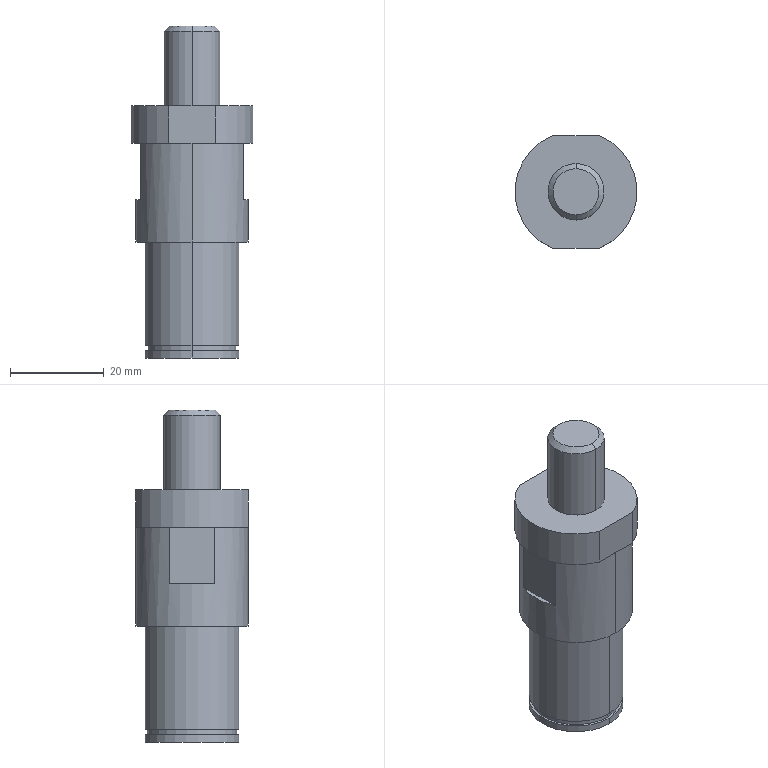Part | STEP file | TNSN20-Y20-F22-Part-2-1 | 1 solid | 28 faces | box 26 x 24 x 70.7 mm | volume 23111 mm3 | plane 14 | cylinder 12 | cone 2 | commonest cylinder face diameters 20 x4 12 x2 19 x2 24 x2 26 x2
STEP:
#1=CARTESIAN_POINT('',(14072.745,13708.046,9.));
#2=VERTEX_POINT('',#1);
#3=CARTESIAN_POINT('',(14072.745,13732.046,9.));
#4=VERTEX_POINT('',#3);
#5=CARTESIAN_POINT('',(14077.745,13720.046,9.));
#6=DIRECTION('',(0.,0.,-1.));
#7=DIRECTION('',(-0.3846,-0.9231,0.));
#8=AXIS2_PLACEMENT_3D('',#5,#6,#7);
#9=CIRCLE('',#8,13.);
#10=EDGE_CURVE('',#2,#4,#9,.T.);
#11=ORIENTED_EDGE('',*,*,#10,.F.);
#12=CARTESIAN_POINT('',(14082.745,13708.046,9.));
#13=VERTEX_POINT('',#12);
#14=CARTESIAN_POINT('',(14082.745,13708.046,9.));
#15=DIRECTION('',(-1.,0.,0.));
#16=VECTOR('',#15,1000.);
#17=LINE('',#14,#16);
#18=EDGE_CURVE('',#13,#2,#17,.T.);
#19=ORIENTED_EDGE('',*,*,#18,.F.);
#20=CARTESIAN_POINT('',(14082.745,13732.046,9.));
#21=VERTEX_POINT('',#20);
#22=CARTESIAN_POINT('',(14077.745,13720.046,9.));
#23=DIRECTION('',(0.,0.,-1.));
#24=DIRECTION('',(0.3846,0.9231,0.));
#25=AXIS2_PLACEMENT_3D('',#22,#23,#24);
#26=CIRCLE('',#25,13.);
#27=EDGE_CURVE('',#21,#13,#26,.T.);
#28=ORIENTED_EDGE('',*,*,#27,.F.);
#29=CARTESIAN_POINT('',(14072.745,13732.046,9.));
#30=DIRECTION('',(1.,0.,0.));
#31=VECTOR('',#30,1000.);
#32=LINE('',#29,#31);
#33=EDGE_CURVE('',#4,#21,#32,.T.);
#34=ORIENTED_EDGE('',*,*,#33,.F.);
#35=EDGE_LOOP('',(#11,#19,#28,#34));
#36=FACE_OUTER_BOUND('',#35,.T.);
#37=CARTESIAN_POINT('',(14077.745,13714.046,9.));
#38=VERTEX_POINT('',#37);
#39=CARTESIAN_POINT('',(14077.745,13726.046,9.));
#40=VERTEX_POINT('',#39);
#41=CARTESIAN_POINT('',(14077.745,13720.046,9.));
#42=DIRECTION('',(0.,0.,-1.));
#43=DIRECTION('',(0.,-1.,0.));
#44=AXIS2_PLACEMENT_3D('',#41,#42,#43);
#45=CIRCLE('',#44,6.);
#46=EDGE_CURVE('',#38,#40,#45,.T.);
#47=ORIENTED_EDGE('',*,*,#46,.T.);
#48=CARTESIAN_POINT('',(14077.745,13720.046,9.));
#49=DIRECTION('',(0.,0.,-1.));
#50=DIRECTION('',(0.,-1.,0.));
#51=AXIS2_PLACEMENT_3D('',#48,#49,#50);
#52=CIRCLE('',#51,6.);
#53=EDGE_CURVE('',#40,#38,#52,.T.);
#54=ORIENTED_EDGE('',*,*,#53,.T.);
#55=EDGE_LOOP('',(#47,#54));
#56=FACE_BOUND('',#55,.T.);
#57=CARTESIAN_POINT('',(14104.283,13746.584,9.));
#58=DIRECTION('',(0.,0.,-1.));
#59=DIRECTION('',(0.,-1.,0.));
#60=AXIS2_PLACEMENT_3D('',#57,#58,#59);
#61=PLANE('',#60);
#62=ADVANCED_FACE('',(#36,#56),#61,.F.);
#63=CARTESIAN_POINT('',(14082.745,13708.046,1.));
#64=VERTEX_POINT('',#63);
#65=CARTESIAN_POINT('',(14082.745,13708.046,9.));
#66=DIRECTION('',(0.,0.,-1.));
#67=VECTOR('',#66,1000.);
#68=LINE('',#65,#67);
#69=EDGE_CURVE('',#13,#64,#68,.T.);
#70=ORIENTED_EDGE('',*,*,#69,.T.);
#71=CARTESIAN_POINT('',(14082.745,13732.046,1.));
#72=VERTEX_POINT('',#71);
#73=CARTESIAN_POINT('',(14077.745,13720.046,1.));
#74=DIRECTION('',(0.,0.,-1.));
#75=DIRECTION('',(0.3846,0.9231,0.));
#76=AXIS2_PLACEMENT_3D('',#73,#74,#75);
#77=CIRCLE('',#76,13.);
#78=EDGE_CURVE('',#72,#64,#77,.T.);
#79=ORIENTED_EDGE('',*,*,#78,.F.);
#80=CARTESIAN_POINT('',(14082.745,13732.046,9.));
#81=DIRECTION('',(0.,0.,-1.));
#82=VECTOR('',#81,1000.);
#83=LINE('',#80,#82);
#84=EDGE_CURVE('',#21,#72,#83,.T.);
#85=ORIENTED_EDGE('',*,*,#84,.F.);
#86=ORIENTED_EDGE('',*,*,#27,.T.);
#87=EDGE_LOOP('',(#70,#79,#85,#86));
#88=FACE_OUTER_BOUND('',#87,.T.);
#89=CARTESIAN_POINT('',(14077.745,13720.046,5.));
#90=DIRECTION('',(0.,0.,-1.));
#91=DIRECTION('',(0.,-1.,0.));
#92=AXIS2_PLACEMENT_3D('',#89,#90,#91);
#93=CYLINDRICAL_SURFACE('',#92,13.);
#94=ADVANCED_FACE('',(#88),#93,.T.);
#95=CARTESIAN_POINT('',(14072.745,13732.046,1.));
#96=VERTEX_POINT('',#95);
#97=CARTESIAN_POINT('',(14072.745,13732.046,9.));
#98=DIRECTION('',(0.,0.,-1.));
#99=VECTOR('',#98,1000.);
#100=LINE('',#97,#99);
#101=EDGE_CURVE('',#4,#96,#100,.T.);
#102=ORIENTED_EDGE('',*,*,#101,.T.);
#103=CARTESIAN_POINT('',(14072.745,13708.046,1.));
#104=VERTEX_POINT('',#103);
#105=CARTESIAN_POINT('',(14077.745,13720.046,1.));
#106=DIRECTION('',(0.,0.,-1.));
#107=DIRECTION('',(-0.3846,-0.9231,0.));
#108=AXIS2_PLACEMENT_3D('',#105,#106,#107);
#109=CIRCLE('',#108,13.);
#110=EDGE_CURVE('',#104,#96,#109,.T.);
#111=ORIENTED_EDGE('',*,*,#110,.F.);
#112=CARTESIAN_POINT('',(14072.745,13708.046,9.));
#113=DIRECTION('',(0.,0.,-1.));
#114=VECTOR('',#113,1000.);
#115=LINE('',#112,#114);
#116=EDGE_CURVE('',#2,#104,#115,.T.);
#117=ORIENTED_EDGE('',*,*,#116,.F.);
#118=ORIENTED_EDGE('',*,*,#10,.T.);
#119=EDGE_LOOP('',(#102,#111,#117,#118));
#120=FACE_OUTER_BOUND('',#119,.T.);
#121=CARTESIAN_POINT('',(14077.745,13720.046,5.));
#122=DIRECTION('',(0.,0.,-1.));
#123=DIRECTION('',(0.,-1.,0.));
#124=AXIS2_PLACEMENT_3D('',#121,#122,#123);
#125=CYLINDRICAL_SURFACE('',#124,13.);
#126=ADVANCED_FACE('',(#120),#125,.T.);
#127=ORIENTED_EDGE('',*,*,#78,.T.);
#128=CARTESIAN_POINT('',(14077.745,13708.046,1.));
#129=VERTEX_POINT('',#128);
#130=CARTESIAN_POINT('',(14082.745,13708.046,1.));
#131=DIRECTION('',(-1.,0.,0.));
#132=VECTOR('',#131,1000.);
#133=LINE('',#130,#132);
#134=EDGE_CURVE('',#64,#129,#133,.T.);
#135=ORIENTED_EDGE('',*,*,#134,.T.);
#136=CARTESIAN_POINT('',(14088.745,13715.25,1.));
#137=VERTEX_POINT('',#136);
#138=CARTESIAN_POINT('',(14077.745,13720.046,1.));
#139=DIRECTION('',(0.,0.,-1.));
#140=DIRECTION('',(0.9167,-0.3997,0.));
#141=AXIS2_PLACEMENT_3D('',#138,#139,#140);
#142=CIRCLE('',#141,12.);
#143=EDGE_CURVE('',#137,#129,#142,.T.);
#144=ORIENTED_EDGE('',*,*,#143,.F.);
#145=CARTESIAN_POINT('',(14088.745,13724.842,1.));
#146=VERTEX_POINT('',#145);
#147=CARTESIAN_POINT('',(14088.745,13724.842,1.));
#148=DIRECTION('',(0.,-1.,0.));
#149=VECTOR('',#148,1000.);
#150=LINE('',#147,#149);
#151=EDGE_CURVE('',#146,#137,#150,.T.);
#152=ORIENTED_EDGE('',*,*,#151,.F.);
#153=CARTESIAN_POINT('',(14077.745,13732.046,1.));
#154=VERTEX_POINT('',#153);
#155=CARTESIAN_POINT('',(14077.745,13720.046,1.));
#156=DIRECTION('',(0.,0.,-1.));
#157=DIRECTION('',(0.,1.,0.));
#158=AXIS2_PLACEMENT_3D('',#155,#156,#157);
#159=CIRCLE('',#158,12.);
#160=EDGE_CURVE('',#154,#146,#159,.T.);
#161=ORIENTED_EDGE('',*,*,#160,.F.);
#162=CARTESIAN_POINT('',(14077.745,13732.046,1.));
#163=DIRECTION('',(1.,0.,0.));
#164=VECTOR('',#163,1000.);
#165=LINE('',#162,#164);
#166=EDGE_CURVE('',#154,#72,#165,.T.);
#167=ORIENTED_EDGE('',*,*,#166,.T.);
#168=EDGE_LOOP('',(#127,#135,#144,#152,#161,#167));
#169=FACE_OUTER_BOUND('',#168,.T.);
#170=CARTESIAN_POINT('',(14104.716,13699.575,1.));
#171=DIRECTION('',(0.,0.,1.));
#172=DIRECTION('',(0.,1.,0.));
#173=AXIS2_PLACEMENT_3D('',#170,#171,#172);
#174=PLANE('',#173);
#175=ADVANCED_FACE('',(#169),#174,.F.);
#176=ORIENTED_EDGE('',*,*,#110,.T.);
#177=CARTESIAN_POINT('',(14072.745,13732.046,1.));
#178=DIRECTION('',(1.,0.,0.));
#179=VECTOR('',#178,1000.);
#180=LINE('',#177,#179);
#181=EDGE_CURVE('',#96,#154,#180,.T.);
#182=ORIENTED_EDGE('',*,*,#181,.T.);
#183=CARTESIAN_POINT('',(14066.745,13724.842,1.));
#184=VERTEX_POINT('',#183);
#185=CARTESIAN_POINT('',(14077.745,13720.046,1.));
#186=DIRECTION('',(0.,0.,-1.));
#187=DIRECTION('',(-0.9167,0.3997,0.));
#188=AXIS2_PLACEMENT_3D('',#185,#186,#187);
#189=CIRCLE('',#188,12.);
#190=EDGE_CURVE('',#184,#154,#189,.T.);
#191=ORIENTED_EDGE('',*,*,#190,.F.);
#192=CARTESIAN_POINT('',(14066.745,13715.25,1.));
#193=VERTEX_POINT('',#192);
#194=CARTESIAN_POINT('',(14066.745,13724.842,1.));
#195=DIRECTION('',(0.,-1.,0.));
#196=VECTOR('',#195,1000.);
#197=LINE('',#194,#196);
#198=EDGE_CURVE('',#184,#193,#197,.T.);
#199=ORIENTED_EDGE('',*,*,#198,.T.);
#200=CARTESIAN_POINT('',(14077.745,13720.046,1.));
#201=DIRECTION('',(0.,0.,-1.));
#202=DIRECTION('',(0.,-1.,0.));
#203=AXIS2_PLACEMENT_3D('',#200,#201,#202);
#204=CIRCLE('',#203,12.);
#205=EDGE_CURVE('',#129,#193,#204,.T.);
#206=ORIENTED_EDGE('',*,*,#205,.F.);
#207=CARTESIAN_POINT('',(14077.745,13708.046,1.));
#208=DIRECTION('',(-1.,0.,0.));
#209=VECTOR('',#208,1000.);
#210=LINE('',#207,#209);
#211=EDGE_CURVE('',#129,#104,#210,.T.);
#212=ORIENTED_EDGE('',*,*,#211,.T.);
#213=EDGE_LOOP('',(#176,#182,#191,#199,#206,#212));
#214=FACE_OUTER_BOUND('',#213,.T.);
#215=CARTESIAN_POINT('',(14091.716,13699.575,1.));
#216=DIRECTION('',(0.,0.,1.));
#217=DIRECTION('',(0.,1.,0.));
#218=AXIS2_PLACEMENT_3D('',#215,#216,#217);
#219=PLANE('',#218);
#220=ADVANCED_FACE('',(#214),#219,.F.);
#221=CARTESIAN_POINT('',(14077.745,13724.973,26.));
#222=VERTEX_POINT('',#221);
#223=CARTESIAN_POINT('',(14077.745,13715.12,26.));
#224=VERTEX_POINT('',#223);
#225=CARTESIAN_POINT('',(14077.745,13720.046,26.));
#226=DIRECTION('',(0.,0.,-1.));
#227=DIRECTION('',(0.,-1.,0.));
#228=AXIS2_PLACEMENT_3D('',#225,#226,#227);
#229=CIRCLE('',#228,4.926);
#230=EDGE_CURVE('',#222,#224,#229,.T.);
#231=ORIENTED_EDGE('',*,*,#230,.F.);
#232=CARTESIAN_POINT('',(14077.745,13720.046,26.));
#233=DIRECTION('',(0.,0.,-1.));
#234=DIRECTION('',(0.,-1.,0.));
#235=AXIS2_PLACEMENT_3D('',#232,#233,#234);
#236=CIRCLE('',#235,4.926);
#237=EDGE_CURVE('',#224,#222,#236,.T.);
#238=ORIENTED_EDGE('',*,*,#237,.F.);
#239=EDGE_LOOP('',(#231,#238));
#240=FACE_OUTER_BOUND('',#239,.T.);
#241=CARTESIAN_POINT('',(14094.677,13739.442,26.));
#242=DIRECTION('',(0.,0.,-1.));
#243=DIRECTION('',(0.,-1.,0.));
#244=AXIS2_PLACEMENT_3D('',#241,#242,#243);
#245=PLANE('',#244);
#246=ADVANCED_FACE('',(#240),#245,.F.);
#247=CARTESIAN_POINT('',(14077.745,13708.046,-20.));
#248=VERTEX_POINT('',#247);
#249=CARTESIAN_POINT('',(14077.745,13732.046,-20.));
#250=VERTEX_POINT('',#249);
#251=CARTESIAN_POINT('',(14077.745,13720.046,-20.));
#252=DIRECTION('',(0.,0.,-1.));
#253=DIRECTION('',(0.,-1.,0.));
#254=AXIS2_PLACEMENT_3D('',#251,#252,#253);
#255=CIRCLE('',#254,12.);
#256=EDGE_CURVE('',#248,#250,#255,.T.);
#257=ORIENTED_EDGE('',*,*,#256,.T.);
#258=CARTESIAN_POINT('',(14077.745,13720.046,-20.));
#259=DIRECTION('',(0.,0.,-1.));
#260=DIRECTION('',(0.,-1.,0.));
#261=AXIS2_PLACEMENT_3D('',#258,#259,#260);
#262=CIRCLE('',#261,12.);
#263=EDGE_CURVE('',#250,#248,#262,.T.);
#264=ORIENTED_EDGE('',*,*,#263,.T.);
#265=EDGE_LOOP('',(#257,#264));
#266=FACE_OUTER_BOUND('',#265,.T.);
#267=CARTESIAN_POINT('',(14077.745,13730.046,-20.));
#268=VERTEX_POINT('',#267);
#269=CARTESIAN_POINT('',(14077.745,13710.046,-20.));
#270=VERTEX_POINT('',#269);
#271=CARTESIAN_POINT('',(14077.745,13720.046,-20.));
#272=DIRECTION('',(0.,0.,-1.));
#273=DIRECTION('',(0.,-1.,0.));
#274=AXIS2_PLACEMENT_3D('',#271,#272,#273);
#275=CIRCLE('',#274,10.);
#276=EDGE_CURVE('',#268,#270,#275,.T.);
#277=ORIENTED_EDGE('',*,*,#276,.F.);
#278=CARTESIAN_POINT('',(14077.745,13720.046,-20.));
#279=DIRECTION('',(0.,0.,-1.));
#280=DIRECTION('',(0.,-1.,0.));
#281=AXIS2_PLACEMENT_3D('',#278,#279,#280);
#282=CIRCLE('',#281,10.);
#283=EDGE_CURVE('',#270,#268,#282,.T.);
#284=ORIENTED_EDGE('',*,*,#283,.F.);
#285=EDGE_LOOP('',(#277,#284));
#286=FACE_BOUND('',#285,.T.);
#287=CARTESIAN_POINT('',(14118.988,13684.803,-20.));
#288=DIRECTION('',(0.,0.,1.));
#289=DIRECTION('',(0.,1.,0.));
#290=AXIS2_PLACEMENT_3D('',#287,#288,#289);
#291=PLANE('',#290);
#292=ADVANCED_FACE('',(#266,#286),#291,.F.);
#293=CARTESIAN_POINT('',(14077.745,13710.046,-42.));
#294=VERTEX_POINT('',#293);
#295=CARTESIAN_POINT('',(14077.745,13730.046,-42.));
#296=VERTEX_POINT('',#295);
#297=CARTESIAN_POINT('',(14077.745,13720.046,-42.));
#298=DIRECTION('',(0.,0.,-1.));
#299=DIRECTION('',(0.,-1.,0.));
#300=AXIS2_PLACEMENT_3D('',#297,#298,#299);
#301=CIRCLE('',#300,10.);
#302=EDGE_CURVE('',#294,#296,#301,.T.);
#303=ORIENTED_EDGE('',*,*,#302,.T.);
#304=CARTESIAN_POINT('',(14077.745,13720.046,-42.));
#305=DIRECTION('',(0.,0.,-1.));
#306=DIRECTION('',(0.,-1.,0.));
#307=AXIS2_PLACEMENT_3D('',#304,#305,#306);
#308=CIRCLE('',#307,10.);
#309=EDGE_CURVE('',#296,#294,#308,.T.);
#310=ORIENTED_EDGE('',*,*,#309,.T.);
#311=EDGE_LOOP('',(#303,#310));
#312=FACE_OUTER_BOUND('',#311,.T.);
#313=CARTESIAN_POINT('',(14077.745,13729.546,-42.));
#314=VERTEX_POINT('',#313);
#315=CARTESIAN_POINT('',(14077.745,13710.546,-42.));
#316=VERTEX_POINT('',#315);
#317=CARTESIAN_POINT('',(14077.745,13720.046,-42.));
#318=DIRECTION('',(0.,0.,-1.));
#319=DIRECTION('',(0.,-1.,0.));
#320=AXIS2_PLACEMENT_3D('',#317,#318,#319);
#321=CIRCLE('',#320,9.5);
#322=EDGE_CURVE('',#314,#316,#321,.T.);
#323=ORIENTED_EDGE('',*,*,#322,.F.);
#324=CARTESIAN_POINT('',(14077.745,13720.046,-42.));
#325=DIRECTION('',(0.,0.,-1.));
#326=DIRECTION('',(0.,-1.,0.));
#327=AXIS2_PLACEMENT_3D('',#324,#325,#326);
#328=CIRCLE('',#327,9.5);
#329=EDGE_CURVE('',#316,#314,#328,.T.);
#330=ORIENTED_EDGE('',*,*,#329,.F.);
#331=EDGE_LOOP('',(#323,#330));
#332=FACE_BOUND('',#331,.T.);
#333=CARTESIAN_POINT('',(14112.114,13690.677,-42.));
#334=DIRECTION('',(0.,0.,1.));
#335=DIRECTION('',(0.,1.,0.));
#336=AXIS2_PLACEMENT_3D('',#333,#334,#335);
#337=PLANE('',#336);
#338=ADVANCED_FACE('',(#312,#332),#337,.F.);
#339=CARTESIAN_POINT('',(14077.745,13730.046,-43.2));
#340=VERTEX_POINT('',#339);
#341=CARTESIAN_POINT('',(14077.745,13710.046,-43.2));
#342=VERTEX_POINT('',#341);
#343=CARTESIAN_POINT('',(14077.745,13720.046,-43.2));
#344=DIRECTION('',(0.,0.,-1.));
#345=DIRECTION('',(0.,-1.,0.));
#346=AXIS2_PLACEMENT_3D('',#343,#344,#345);
#347=CIRCLE('',#346,10.);
#348=EDGE_CURVE('',#340,#342,#347,.T.);
#349=ORIENTED_EDGE('',*,*,#348,.F.);
#350=CARTESIAN_POINT('',(14077.745,13720.046,-43.2));
#351=DIRECTION('',(0.,0.,-1.));
#352=DIRECTION('',(0.,-1.,0.));
#353=AXIS2_PLACEMENT_3D('',#350,#351,#352);
#354=CIRCLE('',#353,10.);
#355=EDGE_CURVE('',#342,#340,#354,.T.);
#356=ORIENTED_EDGE('',*,*,#355,.F.);
#357=EDGE_LOOP('',(#349,#356));
#358=FACE_OUTER_BOUND('',#357,.T.);
#359=CARTESIAN_POINT('',(14077.745,13710.546,-43.2));
#360=VERTEX_POINT('',#359);
#361=CARTESIAN_POINT('',(14077.745,13729.546,-43.2));
#362=VERTEX_POINT('',#361);
#363=CARTESIAN_POINT('',(14077.745,13720.046,-43.2));
#364=DIRECTION('',(0.,0.,-1.));
#365=DIRECTION('',(0.,-1.,0.));
#366=AXIS2_PLACEMENT_3D('',#363,#364,#365);
#367=CIRCLE('',#366,9.5);
#368=EDGE_CURVE('',#360,#362,#367,.T.);
#369=ORIENTED_EDGE('',*,*,#368,.T.);
#370=CARTESIAN_POINT('',(14077.745,13720.046,-43.2));
#371=DIRECTION('',(0.,0.,-1.));
#372=DIRECTION('',(0.,-1.,0.));
#373=AXIS2_PLACEMENT_3D('',#370,#371,#372);
#374=CIRCLE('',#373,9.5);
#375=EDGE_CURVE('',#362,#360,#374,.T.);
#376=ORIENTED_EDGE('',*,*,#375,.T.);
#377=EDGE_LOOP('',(#369,#376));
#378=FACE_BOUND('',#377,.T.);
#379=CARTESIAN_POINT('',(14112.114,13759.416,-43.2));
#380=DIRECTION('',(0.,0.,-1.));
#381=DIRECTION('',(0.,-1.,0.));
#382=AXIS2_PLACEMENT_3D('',#379,#380,#381);
#383=PLANE('',#382);
#384=ADVANCED_FACE('',(#358,#378),#383,.F.);
#385=CARTESIAN_POINT('',(14077.745,13710.046,-44.7));
#386=VERTEX_POINT('',#385);
#387=CARTESIAN_POINT('',(14077.745,13730.046,-44.7));
#388=VERTEX_POINT('',#387);
#389=CARTESIAN_POINT('',(14077.745,13720.046,-44.7));
#390=DIRECTION('',(0.,0.,-1.));
#391=DIRECTION('',(0.,-1.,0.));
#392=AXIS2_PLACEMENT_3D('',#389,#390,#391);
#393=CIRCLE('',#392,10.);
#394=EDGE_CURVE('',#386,#388,#393,.T.);
#395=ORIENTED_EDGE('',*,*,#394,.T.);
#396=CARTESIAN_POINT('',(14077.745,13720.046,-44.7));
#397=DIRECTION('',(0.,0.,-1.));
#398=DIRECTION('',(0.,-1.,0.));
#399=AXIS2_PLACEMENT_3D('',#396,#397,#398);
#400=CIRCLE('',#399,10.);
#401=EDGE_CURVE('',#388,#386,#400,.T.);
#402=ORIENTED_EDGE('',*,*,#401,.T.);
#403=EDGE_LOOP('',(#395,#402));
#404=FACE_OUTER_BOUND('',#403,.T.);
#405=CARTESIAN_POINT('',(14112.114,13690.677,-44.7));
#406=DIRECTION('',(0.,0.,1.));
#407=DIRECTION('',(0.,1.,0.));
#408=AXIS2_PLACEMENT_3D('',#405,#406,#407);
#409=PLANE('',#408);
#410=ADVANCED_FACE('',(#404),#409,.F.);
#411=ORIENTED_EDGE('',*,*,#181,.F.);
#412=ORIENTED_EDGE('',*,*,#101,.F.);
#413=ORIENTED_EDGE('',*,*,#33,.T.);
#414=ORIENTED_EDGE('',*,*,#84,.T.);
#415=ORIENTED_EDGE('',*,*,#166,.F.);
#416=EDGE_LOOP('',(#411,#412,#413,#414,#415));
#417=FACE_OUTER_BOUND('',#416,.T.);
#418=CARTESIAN_POINT('',(14087.35,13732.046,14.605));
#419=DIRECTION('',(0.,1.,0.));
#420=DIRECTION('',(0.,0.,-1.));
#421=AXIS2_PLACEMENT_3D('',#418,#419,#420);
#422=PLANE('',#421);
#423=ADVANCED_FACE('',(#417),#422,.T.);
#424=ORIENTED_EDGE('',*,*,#134,.F.);
#425=ORIENTED_EDGE('',*,*,#69,.F.);
#426=ORIENTED_EDGE('',*,*,#18,.T.);
#427=ORIENTED_EDGE('',*,*,#116,.T.);
#428=ORIENTED_EDGE('',*,*,#211,.F.);
#429=EDGE_LOOP('',(#424,#425,#426,#427,#428));
#430=FACE_OUTER_BOUND('',#429,.T.);
#431=CARTESIAN_POINT('',(14087.35,13708.046,-4.605));
#432=DIRECTION('',(0.,-1.,0.));
#433=DIRECTION('',(0.,0.,1.));
#434=AXIS2_PLACEMENT_3D('',#431,#432,#433);
#435=PLANE('',#434);
#436=ADVANCED_FACE('',(#430),#435,.T.);
#437=CARTESIAN_POINT('',(14066.745,13724.842,-11.));
#438=VERTEX_POINT('',#437);
#439=CARTESIAN_POINT('',(14066.745,13724.842,1.));
#440=DIRECTION('',(0.,0.,-1.));
#441=VECTOR('',#440,1000.);
#442=LINE('',#439,#441);
#443=EDGE_CURVE('',#184,#438,#442,.T.);
#444=ORIENTED_EDGE('',*,*,#443,.T.);
#445=CARTESIAN_POINT('',(14066.745,13715.25,-11.));
#446=VERTEX_POINT('',#445);
#447=CARTESIAN_POINT('',(14066.745,13724.842,-11.));
#448=DIRECTION('',(0.,-1.,0.));
#449=VECTOR('',#448,1000.);
#450=LINE('',#447,#449);
#451=EDGE_CURVE('',#438,#446,#450,.T.);
#452=ORIENTED_EDGE('',*,*,#451,.T.);
#453=CARTESIAN_POINT('',(14066.745,13715.25,1.));
#454=DIRECTION('',(0.,0.,-1.));
#455=VECTOR('',#454,1000.);
#456=LINE('',#453,#455);
#457=EDGE_CURVE('',#193,#446,#456,.T.);
#458=ORIENTED_EDGE('',*,*,#457,.F.);
#459=ORIENTED_EDGE('',*,*,#198,.F.);
#460=EDGE_LOOP('',(#444,#452,#458,#459));
#461=FACE_OUTER_BOUND('',#460,.T.);
#462=CARTESIAN_POINT('',(14066.745,13708.525,6.522));
#463=DIRECTION('',(-1.,0.,0.));
#464=DIRECTION('',(0.,1.,0.));
#465=AXIS2_PLACEMENT_3D('',#462,#463,#464);
#466=PLANE('',#465);
#467=ADVANCED_FACE('',(#461),#466,.T.);
#468=ORIENTED_EDGE('',*,*,#451,.F.);
#469=CARTESIAN_POINT('',(14077.745,13720.046,-11.));
#470=DIRECTION('',(0.,0.,1.));
#471=DIRECTION('',(-0.9167,0.3997,0.));
#472=AXIS2_PLACEMENT_3D('',#469,#470,#471);
#473=CIRCLE('',#472,12.);
#474=EDGE_CURVE('',#438,#446,#473,.T.);
#475=ORIENTED_EDGE('',*,*,#474,.T.);
#476=EDGE_LOOP('',(#468,#475));
#477=FACE_OUTER_BOUND('',#476,.T.);
#478=CARTESIAN_POINT('',(14073.062,13712.684,-11.));
#479=DIRECTION('',(0.,0.,1.));
#480=DIRECTION('',(0.,1.,0.));
#481=AXIS2_PLACEMENT_3D('',#478,#479,#480);
#482=PLANE('',#481);
#483=ADVANCED_FACE('',(#477),#482,.T.);
#484=CARTESIAN_POINT('',(14088.745,13724.842,-11.));
#485=VERTEX_POINT('',#484);
#486=CARTESIAN_POINT('',(14088.745,13715.25,-11.));
#487=VERTEX_POINT('',#486);
#488=CARTESIAN_POINT('',(14088.745,13724.842,-11.));
#489=DIRECTION('',(0.,-1.,0.));
#490=VECTOR('',#489,1000.);
#491=LINE('',#488,#490);
#492=EDGE_CURVE('',#485,#487,#491,.T.);
#493=ORIENTED_EDGE('',*,*,#492,.T.);
#494=CARTESIAN_POINT('',(14077.745,13720.046,-11.));
#495=DIRECTION('',(0.,0.,1.));
#496=DIRECTION('',(0.9167,-0.3997,0.));
#497=AXIS2_PLACEMENT_3D('',#494,#495,#496);
#498=CIRCLE('',#497,12.);
#499=EDGE_CURVE('',#487,#485,#498,.T.);
#500=ORIENTED_EDGE('',*,*,#499,.T.);
#501=EDGE_LOOP('',(#493,#500));
#502=FACE_OUTER_BOUND('',#501,.T.);
#503=CARTESIAN_POINT('',(14097.153,13712.684,-11.));
#504=DIRECTION('',(0.,0.,1.));
#505=DIRECTION('',(0.,1.,0.));
#506=AXIS2_PLACEMENT_3D('',#503,#504,#505);
#507=PLANE('',#506);
#508=ADVANCED_FACE('',(#502),#507,.T.);
#509=CARTESIAN_POINT('',(14088.745,13715.25,1.));
#510=DIRECTION('',(0.,0.,-1.));
#511=VECTOR('',#510,1000.);
#512=LINE('',#509,#511);
#513=EDGE_CURVE('',#137,#487,#512,.T.);
#514=ORIENTED_EDGE('',*,*,#513,.T.);
#515=ORIENTED_EDGE('',*,*,#492,.F.);
#516=CARTESIAN_POINT('',(14088.745,13724.842,1.));
#517=DIRECTION('',(0.,0.,-1.));
#518=VECTOR('',#517,1000.);
#519=LINE('',#516,#518);
#520=EDGE_CURVE('',#146,#485,#519,.T.);
#521=ORIENTED_EDGE('',*,*,#520,.F.);
#522=ORIENTED_EDGE('',*,*,#151,.T.);
#523=EDGE_LOOP('',(#514,#515,#521,#522));
#524=FACE_OUTER_BOUND('',#523,.T.);
#525=CARTESIAN_POINT('',(14088.745,13731.568,6.522));
#526=DIRECTION('',(1.,0.,0.));
#527=DIRECTION('',(0.,-1.,0.));
#528=AXIS2_PLACEMENT_3D('',#525,#526,#527);
#529=PLANE('',#528);
#530=ADVANCED_FACE('',(#524),#529,.T.);
#531=ORIENTED_EDGE('',*,*,#263,.F.);
#532=CARTESIAN_POINT('',(14077.745,13732.046,1.));
#533=DIRECTION('',(0.,0.,-1.));
#534=VECTOR('',#533,1000.);
#535=LINE('',#532,#534);
#536=EDGE_CURVE('',#154,#250,#535,.T.);
#537=ORIENTED_EDGE('',*,*,#536,.F.);
#538=ORIENTED_EDGE('',*,*,#160,.T.);
#539=ORIENTED_EDGE('',*,*,#520,.T.);
#540=ORIENTED_EDGE('',*,*,#499,.F.);
#541=ORIENTED_EDGE('',*,*,#513,.F.);
#542=ORIENTED_EDGE('',*,*,#143,.T.);
#543=CARTESIAN_POINT('',(14077.745,13708.046,1.));
#544=DIRECTION('',(0.,0.,-1.));
#545=VECTOR('',#544,1000.);
#546=LINE('',#543,#545);
#547=EDGE_CURVE('',#129,#248,#546,.T.);
#548=ORIENTED_EDGE('',*,*,#547,.T.);
#549=EDGE_LOOP('',(#531,#537,#538,#539,#540,#541,#542,#548));
#550=FACE_OUTER_BOUND('',#549,.T.);
#551=CARTESIAN_POINT('',(14077.745,13720.046,-9.5));
#552=DIRECTION('',(0.,0.,-1.));
#553=DIRECTION('',(0.,1.,0.));
#554=AXIS2_PLACEMENT_3D('',#551,#552,#553);
#555=CYLINDRICAL_SURFACE('',#554,12.);
#556=ADVANCED_FACE('',(#550),#555,.T.);
#557=ORIENTED_EDGE('',*,*,#205,.T.);
#558=ORIENTED_EDGE('',*,*,#457,.T.);
#559=ORIENTED_EDGE('',*,*,#474,.F.);
#560=ORIENTED_EDGE('',*,*,#443,.F.);
#561=ORIENTED_EDGE('',*,*,#190,.T.);
#562=ORIENTED_EDGE('',*,*,#536,.T.);
#563=ORIENTED_EDGE('',*,*,#256,.F.);
#564=ORIENTED_EDGE('',*,*,#547,.F.);
#565=EDGE_LOOP('',(#557,#558,#559,#560,#561,#562,#563,#564));
#566=FACE_OUTER_BOUND('',#565,.T.);
#567=CARTESIAN_POINT('',(14077.745,13720.046,-9.5));
#568=DIRECTION('',(0.,0.,-1.));
#569=DIRECTION('',(0.,1.,0.));
#570=AXIS2_PLACEMENT_3D('',#567,#568,#569);
#571=CYLINDRICAL_SURFACE('',#570,12.);
#572=ADVANCED_FACE('',(#566),#571,.T.);
#573=ORIENTED_EDGE('',*,*,#237,.T.);
#574=CARTESIAN_POINT('',(14077.745,13726.046,24.927));
#575=VERTEX_POINT('',#574);
#576=CARTESIAN_POINT('',(14077.745,13726.046,24.927));
#577=DIRECTION('',(0.,-0.7071,0.7071));
#578=VECTOR('',#577,1000.);
#579=LINE('',#576,#578);
#580=EDGE_CURVE('',#575,#222,#579,.T.);
#581=ORIENTED_EDGE('',*,*,#580,.F.);
#582=CARTESIAN_POINT('',(14077.745,13714.046,24.927));
#583=VERTEX_POINT('',#582);
#584=CARTESIAN_POINT('',(14077.745,13720.046,24.927));
#585=DIRECTION('',(0.,0.,-1.));
#586=DIRECTION('',(0.,-1.,0.));
#587=AXIS2_PLACEMENT_3D('',#584,#585,#586);
#588=CIRCLE('',#587,6.);
#589=EDGE_CURVE('',#583,#575,#588,.T.);
#590=ORIENTED_EDGE('',*,*,#589,.F.);
#591=CARTESIAN_POINT('',(14077.745,13714.046,24.927));
#592=DIRECTION('',(0.,0.7071,0.7071));
#593=VECTOR('',#592,1000.);
#594=LINE('',#591,#593);
#595=EDGE_CURVE('',#583,#224,#594,.T.);
#596=ORIENTED_EDGE('',*,*,#595,.T.);
#597=EDGE_LOOP('',(#573,#581,#590,#596));
#598=FACE_OUTER_BOUND('',#597,.T.);
#599=CARTESIAN_POINT('',(14077.745,13720.046,-969.074));
#600=DIRECTION('',(0.,0.,-1.));
#601=DIRECTION('',(0.,1.,0.));
#602=AXIS2_PLACEMENT_3D('',#599,#600,#601);
#603=CONICAL_SURFACE('',#602,1000.,0.7854);
#604=ADVANCED_FACE('',(#598),#603,.T.);
#605=CARTESIAN_POINT('',(14077.745,13720.046,24.927));
#606=DIRECTION('',(0.,0.,-1.));
#607=DIRECTION('',(0.,-1.,0.));
#608=AXIS2_PLACEMENT_3D('',#605,#606,#607);
#609=CIRCLE('',#608,6.);
#610=EDGE_CURVE('',#575,#583,#609,.T.);
#611=ORIENTED_EDGE('',*,*,#610,.F.);
#612=ORIENTED_EDGE('',*,*,#580,.T.);
#613=ORIENTED_EDGE('',*,*,#230,.T.);
#614=ORIENTED_EDGE('',*,*,#595,.F.);
#615=EDGE_LOOP('',(#611,#612,#613,#614));
#616=FACE_OUTER_BOUND('',#615,.T.);
#617=CARTESIAN_POINT('',(14077.745,13720.046,-969.074));
#618=DIRECTION('',(0.,0.,-1.));
#619=DIRECTION('',(0.,1.,0.));
#620=AXIS2_PLACEMENT_3D('',#617,#618,#619);
#621=CONICAL_SURFACE('',#620,1000.,0.7854);
#622=ADVANCED_FACE('',(#616),#621,.T.);
#623=ORIENTED_EDGE('',*,*,#53,.F.);
#624=CARTESIAN_POINT('',(14077.745,13726.046,24.927));
#625=DIRECTION('',(0.,0.,-1.));
#626=VECTOR('',#625,1000.);
#627=LINE('',#624,#626);
#628=EDGE_CURVE('',#575,#40,#627,.T.);
#629=ORIENTED_EDGE('',*,*,#628,.F.);
#630=ORIENTED_EDGE('',*,*,#610,.T.);
#631=CARTESIAN_POINT('',(14077.745,13714.046,24.927));
#632=DIRECTION('',(0.,0.,-1.));
#633=VECTOR('',#632,1000.);
#634=LINE('',#631,#633);
#635=EDGE_CURVE('',#583,#38,#634,.T.);
#636=ORIENTED_EDGE('',*,*,#635,.T.);
#637=EDGE_LOOP('',(#623,#629,#630,#636));
#638=FACE_OUTER_BOUND('',#637,.T.);
#639=CARTESIAN_POINT('',(14077.745,13720.046,16.963));
#640=DIRECTION('',(0.,0.,-1.));
#641=DIRECTION('',(0.,1.,0.));
#642=AXIS2_PLACEMENT_3D('',#639,#640,#641);
#643=CYLINDRICAL_SURFACE('',#642,6.);
#644=ADVANCED_FACE('',(#638),#643,.T.);
#645=ORIENTED_EDGE('',*,*,#589,.T.);
#646=ORIENTED_EDGE('',*,*,#628,.T.);
#647=ORIENTED_EDGE('',*,*,#46,.F.);
#648=ORIENTED_EDGE('',*,*,#635,.F.);
#649=EDGE_LOOP('',(#645,#646,#647,#648));
#650=FACE_OUTER_BOUND('',#649,.T.);
#651=CARTESIAN_POINT('',(14077.745,13720.046,16.963));
#652=DIRECTION('',(0.,0.,-1.));
#653=DIRECTION('',(0.,1.,0.));
#654=AXIS2_PLACEMENT_3D('',#651,#652,#653);
#655=CYLINDRICAL_SURFACE('',#654,6.);
#656=ADVANCED_FACE('',(#650),#655,.T.);
#657=ORIENTED_EDGE('',*,*,#309,.F.);
#658=CARTESIAN_POINT('',(14077.745,13730.046,-20.));
#659=DIRECTION('',(0.,0.,-1.));
#660=VECTOR('',#659,1000.);
#661=LINE('',#658,#660);
#662=EDGE_CURVE('',#268,#296,#661,.T.);
#663=ORIENTED_EDGE('',*,*,#662,.F.);
#664=ORIENTED_EDGE('',*,*,#276,.T.);
#665=CARTESIAN_POINT('',(14077.745,13710.046,-20.));
#666=DIRECTION('',(0.,0.,-1.));
#667=VECTOR('',#666,1000.);
#668=LINE('',#665,#667);
#669=EDGE_CURVE('',#270,#294,#668,.T.);
#670=ORIENTED_EDGE('',*,*,#669,.T.);
#671=EDGE_LOOP('',(#657,#663,#664,#670));
#672=FACE_OUTER_BOUND('',#671,.T.);
#673=CARTESIAN_POINT('',(14077.745,13720.046,-31.));
#674=DIRECTION('',(0.,0.,-1.));
#675=DIRECTION('',(0.,1.,0.));
#676=AXIS2_PLACEMENT_3D('',#673,#674,#675);
#677=CYLINDRICAL_SURFACE('',#676,10.);
#678=ADVANCED_FACE('',(#672),#677,.T.);
#679=ORIENTED_EDGE('',*,*,#283,.T.);
#680=ORIENTED_EDGE('',*,*,#662,.T.);
#681=ORIENTED_EDGE('',*,*,#302,.F.);
#682=ORIENTED_EDGE('',*,*,#669,.F.);
#683=EDGE_LOOP('',(#679,#680,#681,#682));
#684=FACE_OUTER_BOUND('',#683,.T.);
#685=CARTESIAN_POINT('',(14077.745,13720.046,-31.));
#686=DIRECTION('',(0.,0.,-1.));
#687=DIRECTION('',(0.,1.,0.));
#688=AXIS2_PLACEMENT_3D('',#685,#686,#687);
#689=CYLINDRICAL_SURFACE('',#688,10.);
#690=ADVANCED_FACE('',(#684),#689,.T.);
#691=ORIENTED_EDGE('',*,*,#375,.F.);
#692=CARTESIAN_POINT('',(14077.745,13729.546,-42.));
#693=DIRECTION('',(0.,0.,-1.));
#694=VECTOR('',#693,1000.);
#695=LINE('',#692,#694);
#696=EDGE_CURVE('',#314,#362,#695,.T.);
#697=ORIENTED_EDGE('',*,*,#696,.F.);
#698=ORIENTED_EDGE('',*,*,#322,.T.);
#699=CARTESIAN_POINT('',(14077.745,13710.546,-42.));
#700=DIRECTION('',(0.,0.,-1.));
#701=VECTOR('',#700,1000.);
#702=LINE('',#699,#701);
#703=EDGE_CURVE('',#316,#360,#702,.T.);
#704=ORIENTED_EDGE('',*,*,#703,.T.);
#705=EDGE_LOOP('',(#691,#697,#698,#704));
#706=FACE_OUTER_BOUND('',#705,.T.);
#707=CARTESIAN_POINT('',(14077.745,13720.046,-42.6));
#708=DIRECTION('',(0.,0.,-1.));
#709=DIRECTION('',(0.,1.,0.));
#710=AXIS2_PLACEMENT_3D('',#707,#708,#709);
#711=CYLINDRICAL_SURFACE('',#710,9.5);
#712=ADVANCED_FACE('',(#706),#711,.T.);
#713=ORIENTED_EDGE('',*,*,#329,.T.);
#714=ORIENTED_EDGE('',*,*,#696,.T.);
#715=ORIENTED_EDGE('',*,*,#368,.F.);
#716=ORIENTED_EDGE('',*,*,#703,.F.);
#717=EDGE_LOOP('',(#713,#714,#715,#716));
#718=FACE_OUTER_BOUND('',#717,.T.);
#719=CARTESIAN_POINT('',(14077.745,13720.046,-42.6));
#720=DIRECTION('',(0.,0.,-1.));
#721=DIRECTION('',(0.,1.,0.));
#722=AXIS2_PLACEMENT_3D('',#719,#720,#721);
#723=CYLINDRICAL_SURFACE('',#722,9.5);
#724=ADVANCED_FACE('',(#718),#723,.T.);
#725=ORIENTED_EDGE('',*,*,#401,.F.);
#726=CARTESIAN_POINT('',(14077.745,13730.046,-43.2));
#727=DIRECTION('',(0.,0.,-1.));
#728=VECTOR('',#727,1000.);
#729=LINE('',#726,#728);
#730=EDGE_CURVE('',#340,#388,#729,.T.);
#731=ORIENTED_EDGE('',*,*,#730,.F.);
#732=ORIENTED_EDGE('',*,*,#348,.T.);
#733=CARTESIAN_POINT('',(14077.745,13710.046,-43.2));
#734=DIRECTION('',(0.,0.,-1.));
#735=VECTOR('',#734,1000.);
#736=LINE('',#733,#735);
#737=EDGE_CURVE('',#342,#386,#736,.T.);
#738=ORIENTED_EDGE('',*,*,#737,.T.);
#739=EDGE_LOOP('',(#725,#731,#732,#738));
#740=FACE_OUTER_BOUND('',#739,.T.);
#741=CARTESIAN_POINT('',(14077.745,13720.046,-43.95));
#742=DIRECTION('',(0.,0.,-1.));
#743=DIRECTION('',(0.,1.,0.));
#744=AXIS2_PLACEMENT_3D('',#741,#742,#743);
#745=CYLINDRICAL_SURFACE('',#744,10.);
#746=ADVANCED_FACE('',(#740),#745,.T.);
#747=ORIENTED_EDGE('',*,*,#355,.T.);
#748=ORIENTED_EDGE('',*,*,#730,.T.);
#749=ORIENTED_EDGE('',*,*,#394,.F.);
#750=ORIENTED_EDGE('',*,*,#737,.F.);
#751=EDGE_LOOP('',(#747,#748,#749,#750));
#752=FACE_OUTER_BOUND('',#751,.T.);
#753=CARTESIAN_POINT('',(14077.745,13720.046,-43.95));
#754=DIRECTION('',(0.,0.,-1.));
#755=DIRECTION('',(0.,1.,0.));
#756=AXIS2_PLACEMENT_3D('',#753,#754,#755);
#757=CYLINDRICAL_SURFACE('',#756,10.);
#758=ADVANCED_FACE('',(#752),#757,.T.);
#759=CLOSED_SHELL('',(#62,#94,#126,#175,#220,#246,#292,#338,#384,#410,#423,#436,#467,#483,#508,#530,#556,#572,#604,#622,#644,#656,#678,#690,#712,#724,#746,#758));
#760=MANIFOLD_SOLID_BREP('',#759);
#761=CARTESIAN_POINT('',(0.,0.,0.));
#762=DIRECTION('',(0.,0.,1.));
#763=DIRECTION('',(1.,0.,0.));
#764=AXIS2_PLACEMENT_3D('',#761,#762,#763);
#765=(LENGTH_UNIT()NAMED_UNIT(*)SI_UNIT(.MILLI.,.METRE.));
#766=UNCERTAINTY_MEASURE_WITH_UNIT(LENGTH_MEASURE(0.00001),#765,'','');
#767=(NAMED_UNIT(*)PLANE_ANGLE_UNIT()SI_UNIT($,.RADIAN.));
#768=(NAMED_UNIT(*)SI_UNIT($,.STERADIAN.)SOLID_ANGLE_UNIT());
#769=(GEOMETRIC_REPRESENTATION_CONTEXT(3)GLOBAL_UNCERTAINTY_ASSIGNED_CONTEXT((#766))GLOBAL_UNIT_ASSIGNED_CONTEXT((#765,#767,#768))REPRESENTATION_CONTEXT('',''));
#770=ADVANCED_BREP_SHAPE_REPRESENTATION('',(#760,#764),#769);